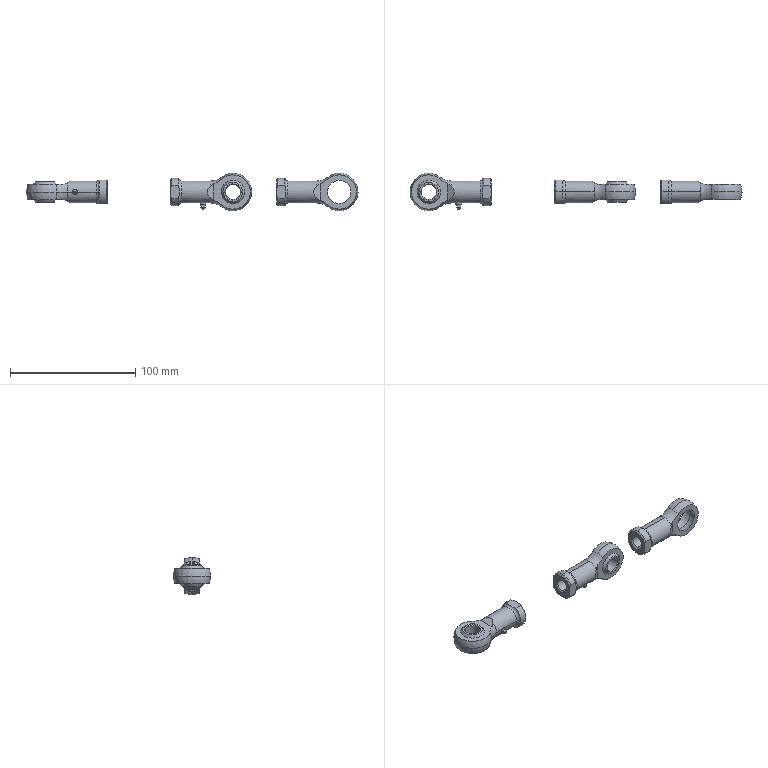Part | NX | 9 solids | 145 faces | box 265.5 x 30 x 30 mm | volume 39780 mm3 | cylinder 43 | plane 34 | cone 29 | sphere 24 | torus 15 | commonest cylinder face diameters 22 x9 10.096 x6 10.106 x6 17.5 x6 1.4 x4 3.5 x4